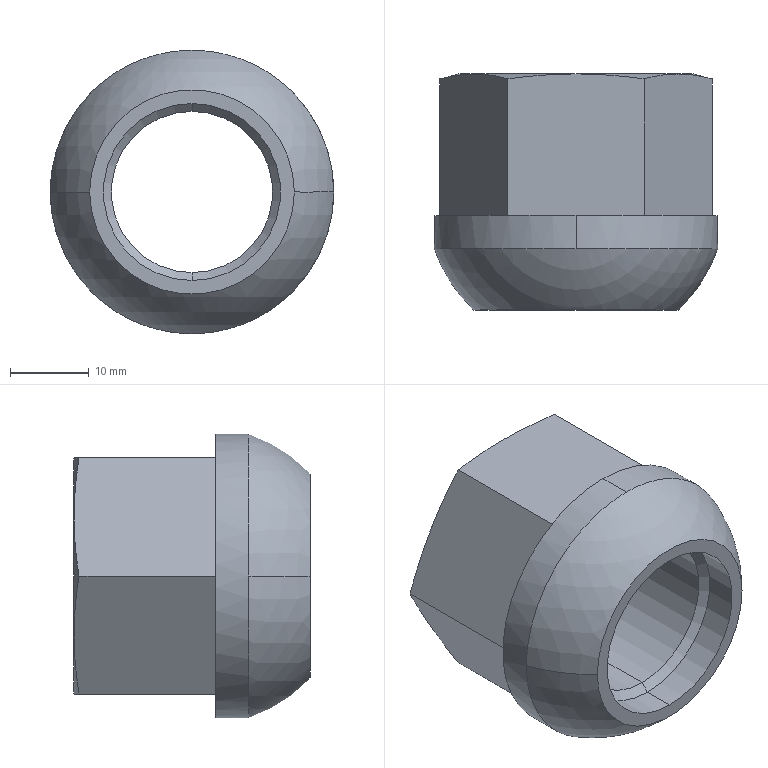Part | SolidWorks | features HoleWzd 1, ICE 1, RevCut 1, Revolution 1 | 1 solid | 21 faces | box 36 x 30 x 36 mm | volume 14362 mm3 | plane 9 | cylinder 6 | cone 4 | sphere 2 | commonest cylinder face diameters 20.5 x2 22.5 x2 36 x2
STEP:
#1=CARTESIAN_POINT('',(0.,30.,-14.928));
#2=VERTEX_POINT('',#1);
#3=CARTESIAN_POINT('',(0.,30.,14.928));
#4=VERTEX_POINT('',#3);
#5=CARTESIAN_POINT('',(0.,30.,0.));
#6=DIRECTION('',(0.,-1.,0.));
#7=DIRECTION('',(0.,0.,1.));
#8=AXIS2_PLACEMENT_3D('',#5,#6,#7);
#9=CIRCLE('',#8,14.928);
#10=EDGE_CURVE('',#2,#4,#9,.T.);
#11=ORIENTED_EDGE('',*,*,#10,.T.);
#12=CARTESIAN_POINT('',(0.,29.981,15.));
#13=VERTEX_POINT('',#12);
#14=CARTESIAN_POINT('',(0.,32.349,6.163));
#15=DIRECTION('',(0.,-0.2588,0.9659));
#16=VECTOR('',#15,1000.);
#17=LINE('',#14,#16);
#18=EDGE_CURVE('',#4,#13,#17,.T.);
#19=ORIENTED_EDGE('',*,*,#18,.T.);
#20=CARTESIAN_POINT('',(8.65,29.36,15.));
#21=VERTEX_POINT('',#20);
#22=CARTESIAN_POINT('',(0.,29.981,15.));
#23=CARTESIAN_POINT('',(1.445,29.981,15.));
#24=CARTESIAN_POINT('',(2.888,29.924,15.));
#25=CARTESIAN_POINT('',(5.771,29.71,15.));
#26=CARTESIAN_POINT('',(7.211,29.553,15.));
#27=CARTESIAN_POINT('',(8.65,29.36,15.));
#28=B_SPLINE_CURVE_WITH_KNOTS('',3,(#22,#23,#24,#25,#26,#27),.UNSPECIFIED.,.F.,.F.,(4,2,4),(0.02331,0.02767,0.03204),.UNSPECIFIED.);
#29=EDGE_CURVE('',#13,#21,#28,.T.);
#30=ORIENTED_EDGE('',*,*,#29,.T.);
#31=CARTESIAN_POINT('',(17.3,29.364,0.));
#32=VERTEX_POINT('',#31);
#33=CARTESIAN_POINT('',(8.65,29.36,15.));
#34=CARTESIAN_POINT('',(9.371,29.554,13.75));
#35=CARTESIAN_POINT('',(10.092,29.711,12.5));
#36=CARTESIAN_POINT('',(11.533,29.927,10.));
#37=CARTESIAN_POINT('',(12.254,29.984,8.75));
#38=CARTESIAN_POINT('',(13.696,29.985,6.25));
#39=CARTESIAN_POINT('',(14.417,29.928,5.));
#40=CARTESIAN_POINT('',(15.858,29.714,2.5));
#41=CARTESIAN_POINT('',(16.579,29.558,1.25));
#42=CARTESIAN_POINT('',(17.3,29.364,0.));
#43=B_SPLINE_CURVE_WITH_KNOTS('',3,(#33,#34,#35,#36,#37,#38,#39,#40,#41,#42),.UNSPECIFIED.,.F.,.F.,(4,2,2,2,4),(0.000000231,0.004329,0.008658,0.01299,0.01732),.UNSPECIFIED.);
#44=EDGE_CURVE('',#21,#32,#43,.T.);
#45=ORIENTED_EDGE('',*,*,#44,.T.);
#46=CARTESIAN_POINT('',(8.65,29.36,-15.));
#47=VERTEX_POINT('',#46);
#48=CARTESIAN_POINT('',(17.3,29.364,0.));
#49=CARTESIAN_POINT('',(16.579,29.558,-1.25));
#50=CARTESIAN_POINT('',(15.858,29.714,-2.5));
#51=CARTESIAN_POINT('',(14.417,29.928,-5.));
#52=CARTESIAN_POINT('',(13.696,29.985,-6.25));
#53=CARTESIAN_POINT('',(12.254,29.984,-8.75));
#54=CARTESIAN_POINT('',(11.533,29.927,-10.));
#55=CARTESIAN_POINT('',(10.092,29.711,-12.5));
#56=CARTESIAN_POINT('',(9.371,29.554,-13.75));
#57=CARTESIAN_POINT('',(8.65,29.36,-15.));
#58=B_SPLINE_CURVE_WITH_KNOTS('',3,(#48,#49,#50,#51,#52,#53,#54,#55,#56,#57),.UNSPECIFIED.,.F.,.F.,(4,2,2,2,4),(0.000000231,0.004329,0.008658,0.01299,0.01732),.UNSPECIFIED.);
#59=EDGE_CURVE('',#32,#47,#58,.T.);
#60=ORIENTED_EDGE('',*,*,#59,.T.);
#61=CARTESIAN_POINT('',(0.,29.981,-15.));
#62=VERTEX_POINT('',#61);
#63=CARTESIAN_POINT('',(8.65,29.36,-15.));
#64=CARTESIAN_POINT('',(7.211,29.553,-15.));
#65=CARTESIAN_POINT('',(5.771,29.71,-15.));
#66=CARTESIAN_POINT('',(2.888,29.924,-15.));
#67=CARTESIAN_POINT('',(1.445,29.981,-15.));
#68=CARTESIAN_POINT('',(0.,29.981,-15.));
#69=B_SPLINE_CURVE_WITH_KNOTS('',3,(#63,#64,#65,#66,#67,#68),.UNSPECIFIED.,.F.,.F.,(4,2,4),(0.03368,0.03804,0.04239),.UNSPECIFIED.);
#70=EDGE_CURVE('',#47,#62,#69,.T.);
#71=ORIENTED_EDGE('',*,*,#70,.T.);
#72=CARTESIAN_POINT('',(0.,32.349,-6.163));
#73=DIRECTION('',(0.,-0.2588,-0.9659));
#74=VECTOR('',#73,1000.);
#75=LINE('',#72,#74);
#76=EDGE_CURVE('',#2,#62,#75,.T.);
#77=ORIENTED_EDGE('',*,*,#76,.F.);
#78=EDGE_LOOP('',(#11,#19,#30,#45,#60,#71,#77));
#79=FACE_OUTER_BOUND('',#78,.T.);
#80=CARTESIAN_POINT('',(0.,32.349,0.));
#81=DIRECTION('',(0.,-1.,0.));
#82=DIRECTION('',(0.,0.,-1.));
#83=AXIS2_PLACEMENT_3D('',#80,#81,#82);
#84=CONICAL_SURFACE('',#83,6.163,1.309);
#85=ADVANCED_FACE('',(#79),#84,.T.);
#86=CARTESIAN_POINT('',(0.,4.96,10.25));
#87=VERTEX_POINT('',#86);
#88=CARTESIAN_POINT('',(0.,4.96,-10.25));
#89=VERTEX_POINT('',#88);
#90=CARTESIAN_POINT('',(0.,4.96,0.));
#91=DIRECTION('',(0.,-1.,0.));
#92=DIRECTION('',(0.,0.,-1.));
#93=AXIS2_PLACEMENT_3D('',#90,#91,#92);
#94=CIRCLE('',#93,10.25);
#95=EDGE_CURVE('',#87,#89,#94,.T.);
#96=ORIENTED_EDGE('',*,*,#95,.T.);
#97=CARTESIAN_POINT('',(0.,30.,-10.25));
#98=VERTEX_POINT('',#97);
#99=CARTESIAN_POINT('',(0.,30.,-10.25));
#100=DIRECTION('',(0.,1.,0.));
#101=VECTOR('',#100,1000.);
#102=LINE('',#99,#101);
#103=EDGE_CURVE('',#89,#98,#102,.T.);
#104=ORIENTED_EDGE('',*,*,#103,.T.);
#105=CARTESIAN_POINT('',(0.,30.,10.25));
#106=VERTEX_POINT('',#105);
#107=CARTESIAN_POINT('',(0.,30.,0.));
#108=DIRECTION('',(0.,1.,0.));
#109=DIRECTION('',(0.,0.,1.));
#110=AXIS2_PLACEMENT_3D('',#107,#108,#109);
#111=CIRCLE('',#110,10.25);
#112=EDGE_CURVE('',#98,#106,#111,.T.);
#113=ORIENTED_EDGE('',*,*,#112,.T.);
#114=CARTESIAN_POINT('',(0.,30.,10.25));
#115=DIRECTION('',(0.,1.,0.));
#116=VECTOR('',#115,1000.);
#117=LINE('',#114,#116);
#118=EDGE_CURVE('',#87,#106,#117,.T.);
#119=ORIENTED_EDGE('',*,*,#118,.F.);
#120=EDGE_LOOP('',(#96,#104,#113,#119));
#121=FACE_OUTER_BOUND('',#120,.T.);
#122=CARTESIAN_POINT('',(0.,30.,0.));
#123=DIRECTION('',(0.,1.,0.));
#124=DIRECTION('',(0.,0.,1.));
#125=AXIS2_PLACEMENT_3D('',#122,#123,#124);
#126=CYLINDRICAL_SURFACE('',#125,10.25);
#127=ADVANCED_FACE('',(#121),#126,.F.);
#128=ORIENTED_EDGE('',*,*,#95,.F.);
#129=CARTESIAN_POINT('',(0.,4.,11.25));
#130=VERTEX_POINT('',#129);
#131=CARTESIAN_POINT('',(0.,4.,11.25));
#132=DIRECTION('',(0.,-0.6925,0.7214));
#133=VECTOR('',#132,1000.);
#134=LINE('',#131,#133);
#135=EDGE_CURVE('',#87,#130,#134,.T.);
#136=ORIENTED_EDGE('',*,*,#135,.T.);
#137=CARTESIAN_POINT('',(0.,4.,-11.25));
#138=VERTEX_POINT('',#137);
#139=CARTESIAN_POINT('',(0.,4.,0.));
#140=DIRECTION('',(0.,1.,0.));
#141=DIRECTION('',(0.,0.,1.));
#142=AXIS2_PLACEMENT_3D('',#139,#140,#141);
#143=CIRCLE('',#142,11.25);
#144=EDGE_CURVE('',#138,#130,#143,.T.);
#145=ORIENTED_EDGE('',*,*,#144,.F.);
#146=CARTESIAN_POINT('',(0.,4.,-11.25));
#147=DIRECTION('',(0.,-0.6925,-0.7214));
#148=VECTOR('',#147,1000.);
#149=LINE('',#146,#148);
#150=EDGE_CURVE('',#89,#138,#149,.T.);
#151=ORIENTED_EDGE('',*,*,#150,.F.);
#152=EDGE_LOOP('',(#128,#136,#145,#151));
#153=FACE_OUTER_BOUND('',#152,.T.);
#154=CARTESIAN_POINT('',(0.,4.,0.));
#155=DIRECTION('',(0.,-1.,0.));
#156=DIRECTION('',(0.,0.,-1.));
#157=AXIS2_PLACEMENT_3D('',#154,#155,#156);
#158=CONICAL_SURFACE('',#157,11.25,0.8058);
#159=ADVANCED_FACE('',(#153),#158,.F.);
#160=CARTESIAN_POINT('',(0.,0.,-11.25));
#161=VERTEX_POINT('',#160);
#162=CARTESIAN_POINT('',(0.,0.,11.25));
#163=VERTEX_POINT('',#162);
#164=CARTESIAN_POINT('',(0.,0.,0.));
#165=DIRECTION('',(0.,1.,0.));
#166=DIRECTION('',(0.,0.,1.));
#167=AXIS2_PLACEMENT_3D('',#164,#165,#166);
#168=CIRCLE('',#167,11.25);
#169=EDGE_CURVE('',#161,#163,#168,.T.);
#170=ORIENTED_EDGE('',*,*,#169,.F.);
#171=CARTESIAN_POINT('',(0.,29.869,-11.25));
#172=DIRECTION('',(0.,1.,0.));
#173=VECTOR('',#172,1000.);
#174=LINE('',#171,#173);
#175=EDGE_CURVE('',#161,#138,#174,.T.);
#176=ORIENTED_EDGE('',*,*,#175,.T.);
#177=ORIENTED_EDGE('',*,*,#144,.T.);
#178=CARTESIAN_POINT('',(0.,29.869,11.25));
#179=DIRECTION('',(0.,1.,0.));
#180=VECTOR('',#179,1000.);
#181=LINE('',#178,#180);
#182=EDGE_CURVE('',#163,#130,#181,.T.);
#183=ORIENTED_EDGE('',*,*,#182,.F.);
#184=EDGE_LOOP('',(#170,#176,#177,#183));
#185=FACE_OUTER_BOUND('',#184,.T.);
#186=CARTESIAN_POINT('',(0.,29.869,0.));
#187=DIRECTION('',(0.,1.,0.));
#188=DIRECTION('',(0.,0.,1.));
#189=AXIS2_PLACEMENT_3D('',#186,#187,#188);
#190=CYLINDRICAL_SURFACE('',#189,11.25);
#191=ADVANCED_FACE('',(#185),#190,.F.);
#192=CARTESIAN_POINT('',(-13.,0.,0.));
#193=VERTEX_POINT('',#192);
#194=CARTESIAN_POINT('',(13.,0.,0.));
#195=VERTEX_POINT('',#194);
#196=CARTESIAN_POINT('',(0.,0.,0.));
#197=DIRECTION('',(0.,1.,0.));
#198=DIRECTION('',(0.,0.,1.));
#199=AXIS2_PLACEMENT_3D('',#196,#197,#198);
#200=CIRCLE('',#199,13.);
#201=EDGE_CURVE('',#193,#195,#200,.T.);
#202=ORIENTED_EDGE('',*,*,#201,.T.);
#203=CARTESIAN_POINT('',(18.,7.774,0.));
#204=VERTEX_POINT('',#203);
#205=CARTESIAN_POINT('',(0.,13.856,0.));
#206=DIRECTION('',(0.,0.,1.));
#207=DIRECTION('',(1.,0.,0.));
#208=AXIS2_PLACEMENT_3D('',#205,#206,#207);
#209=CIRCLE('',#208,19.);
#210=EDGE_CURVE('',#195,#204,#209,.T.);
#211=ORIENTED_EDGE('',*,*,#210,.T.);
#212=CARTESIAN_POINT('',(0.,7.774,18.));
#213=VERTEX_POINT('',#212);
#214=CARTESIAN_POINT('',(0.,7.774,0.));
#215=DIRECTION('',(0.,1.,0.));
#216=DIRECTION('',(0.,0.,1.));
#217=AXIS2_PLACEMENT_3D('',#214,#215,#216);
#218=CIRCLE('',#217,18.);
#219=EDGE_CURVE('',#213,#204,#218,.T.);
#220=ORIENTED_EDGE('',*,*,#219,.F.);
#221=CARTESIAN_POINT('',(-18.,7.774,0.));
#222=VERTEX_POINT('',#221);
#223=CARTESIAN_POINT('',(0.,7.774,0.));
#224=DIRECTION('',(0.,1.,0.));
#225=DIRECTION('',(0.,0.,1.));
#226=AXIS2_PLACEMENT_3D('',#223,#224,#225);
#227=CIRCLE('',#226,18.);
#228=EDGE_CURVE('',#222,#213,#227,.T.);
#229=ORIENTED_EDGE('',*,*,#228,.F.);
#230=CARTESIAN_POINT('',(0.,13.856,0.));
#231=DIRECTION('',(0.,0.,-1.));
#232=DIRECTION('',(-1.,0.,0.));
#233=AXIS2_PLACEMENT_3D('',#230,#231,#232);
#234=CIRCLE('',#233,19.);
#235=EDGE_CURVE('',#193,#222,#234,.T.);
#236=ORIENTED_EDGE('',*,*,#235,.F.);
#237=EDGE_LOOP('',(#202,#211,#220,#229,#236));
#238=FACE_OUTER_BOUND('',#237,.T.);
#239=CARTESIAN_POINT('',(0.,13.856,0.));
#240=DIRECTION('',(0.,0.,1.));
#241=DIRECTION('',(-1.,0.,0.));
#242=AXIS2_PLACEMENT_3D('',#239,#240,#241);
#243=SPHERICAL_SURFACE('',#242,19.);
#244=ADVANCED_FACE('',(#238),#243,.T.);
#245=ORIENTED_EDGE('',*,*,#219,.T.);
#246=CARTESIAN_POINT('',(0.,7.774,-18.));
#247=VERTEX_POINT('',#246);
#248=CARTESIAN_POINT('',(0.,7.774,0.));
#249=DIRECTION('',(0.,1.,0.));
#250=DIRECTION('',(0.,0.,1.));
#251=AXIS2_PLACEMENT_3D('',#248,#249,#250);
#252=CIRCLE('',#251,18.);
#253=EDGE_CURVE('',#204,#247,#252,.T.);
#254=ORIENTED_EDGE('',*,*,#253,.T.);
#255=CARTESIAN_POINT('',(0.,12.,-18.));
#256=VERTEX_POINT('',#255);
#257=CARTESIAN_POINT('',(0.,29.869,-18.));
#258=DIRECTION('',(0.,1.,0.));
#259=VECTOR('',#258,1000.);
#260=LINE('',#257,#259);
#261=EDGE_CURVE('',#247,#256,#260,.T.);
#262=ORIENTED_EDGE('',*,*,#261,.T.);
#263=CARTESIAN_POINT('',(0.,12.,18.));
#264=VERTEX_POINT('',#263);
#265=CARTESIAN_POINT('',(0.,12.,0.));
#266=DIRECTION('',(0.,-1.,0.));
#267=DIRECTION('',(0.,0.,1.));
#268=AXIS2_PLACEMENT_3D('',#265,#266,#267);
#269=CIRCLE('',#268,18.);
#270=EDGE_CURVE('',#256,#264,#269,.T.);
#271=ORIENTED_EDGE('',*,*,#270,.T.);
#272=CARTESIAN_POINT('',(0.,29.869,18.));
#273=DIRECTION('',(0.,1.,0.));
#274=VECTOR('',#273,1000.);
#275=LINE('',#272,#274);
#276=EDGE_CURVE('',#213,#264,#275,.T.);
#277=ORIENTED_EDGE('',*,*,#276,.F.);
#278=EDGE_LOOP('',(#245,#254,#262,#271,#277));
#279=FACE_OUTER_BOUND('',#278,.T.);
#280=CARTESIAN_POINT('',(0.,29.869,0.));
#281=DIRECTION('',(0.,1.,0.));
#282=DIRECTION('',(0.,0.,1.));
#283=AXIS2_PLACEMENT_3D('',#280,#281,#282);
#284=CYLINDRICAL_SURFACE('',#283,18.);
#285=ADVANCED_FACE('',(#279),#284,.T.);
#286=ORIENTED_EDGE('',*,*,#10,.F.);
#287=CARTESIAN_POINT('',(0.,30.,0.));
#288=DIRECTION('',(0.,-1.,0.));
#289=DIRECTION('',(0.,0.,1.));
#290=AXIS2_PLACEMENT_3D('',#287,#288,#289);
#291=CIRCLE('',#290,14.928);
#292=EDGE_CURVE('',#4,#2,#291,.T.);
#293=ORIENTED_EDGE('',*,*,#292,.F.);
#294=EDGE_LOOP('',(#286,#293));
#295=FACE_OUTER_BOUND('',#294,.T.);
#296=CARTESIAN_POINT('',(0.,30.,0.));
#297=DIRECTION('',(0.,1.,0.));
#298=DIRECTION('',(0.,0.,1.));
#299=AXIS2_PLACEMENT_3D('',#296,#297,#298);
#300=CIRCLE('',#299,10.25);
#301=EDGE_CURVE('',#106,#98,#300,.T.);
#302=ORIENTED_EDGE('',*,*,#301,.F.);
#303=ORIENTED_EDGE('',*,*,#112,.F.);
#304=EDGE_LOOP('',(#302,#303));
#305=FACE_BOUND('',#304,.T.);
#306=CARTESIAN_POINT('',(-18.,30.,0.));
#307=DIRECTION('',(0.,1.,0.));
#308=DIRECTION('',(0.,0.,1.));
#309=AXIS2_PLACEMENT_3D('',#306,#307,#308);
#310=PLANE('',#309);
#311=ADVANCED_FACE('',(#295,#305),#310,.T.);
#312=ORIENTED_EDGE('',*,*,#261,.F.);
#313=CARTESIAN_POINT('',(0.,7.774,0.));
#314=DIRECTION('',(0.,1.,0.));
#315=DIRECTION('',(0.,0.,1.));
#316=AXIS2_PLACEMENT_3D('',#313,#314,#315);
#317=CIRCLE('',#316,18.);
#318=EDGE_CURVE('',#247,#222,#317,.T.);
#319=ORIENTED_EDGE('',*,*,#318,.T.);
#320=ORIENTED_EDGE('',*,*,#228,.T.);
#321=ORIENTED_EDGE('',*,*,#276,.T.);
#322=CARTESIAN_POINT('',(0.,12.,0.));
#323=DIRECTION('',(0.,-1.,0.));
#324=DIRECTION('',(0.,0.,1.));
#325=AXIS2_PLACEMENT_3D('',#322,#323,#324);
#326=CIRCLE('',#325,18.);
#327=EDGE_CURVE('',#264,#256,#326,.T.);
#328=ORIENTED_EDGE('',*,*,#327,.T.);
#329=EDGE_LOOP('',(#312,#319,#320,#321,#328));
#330=FACE_OUTER_BOUND('',#329,.T.);
#331=CARTESIAN_POINT('',(0.,29.869,0.));
#332=DIRECTION('',(0.,1.,0.));
#333=DIRECTION('',(0.,0.,1.));
#334=AXIS2_PLACEMENT_3D('',#331,#332,#333);
#335=CYLINDRICAL_SURFACE('',#334,18.);
#336=ADVANCED_FACE('',(#330),#335,.T.);
#337=ORIENTED_EDGE('',*,*,#210,.F.);
#338=CARTESIAN_POINT('',(0.,0.,0.));
#339=DIRECTION('',(0.,1.,0.));
#340=DIRECTION('',(0.,0.,1.));
#341=AXIS2_PLACEMENT_3D('',#338,#339,#340);
#342=CIRCLE('',#341,13.);
#343=EDGE_CURVE('',#195,#193,#342,.T.);
#344=ORIENTED_EDGE('',*,*,#343,.T.);
#345=ORIENTED_EDGE('',*,*,#235,.T.);
#346=ORIENTED_EDGE('',*,*,#318,.F.);
#347=ORIENTED_EDGE('',*,*,#253,.F.);
#348=EDGE_LOOP('',(#337,#344,#345,#346,#347));
#349=FACE_OUTER_BOUND('',#348,.T.);
#350=CARTESIAN_POINT('',(0.,13.856,0.));
#351=DIRECTION('',(0.,0.,1.));
#352=DIRECTION('',(-1.,0.,0.));
#353=AXIS2_PLACEMENT_3D('',#350,#351,#352);
#354=SPHERICAL_SURFACE('',#353,19.);
#355=ADVANCED_FACE('',(#349),#354,.T.);
#356=CARTESIAN_POINT('',(0.,0.,0.));
#357=DIRECTION('',(0.,1.,0.));
#358=DIRECTION('',(0.,0.,1.));
#359=AXIS2_PLACEMENT_3D('',#356,#357,#358);
#360=CIRCLE('',#359,11.25);
#361=EDGE_CURVE('',#163,#161,#360,.T.);
#362=ORIENTED_EDGE('',*,*,#361,.T.);
#363=ORIENTED_EDGE('',*,*,#169,.T.);
#364=EDGE_LOOP('',(#362,#363));
#365=FACE_BOUND('',#364,.T.);
#366=ORIENTED_EDGE('',*,*,#201,.F.);
#367=ORIENTED_EDGE('',*,*,#343,.F.);
#368=EDGE_LOOP('',(#366,#367));
#369=FACE_OUTER_BOUND('',#368,.T.);
#370=CARTESIAN_POINT('',(-13.,0.,0.));
#371=DIRECTION('',(0.,-1.,0.));
#372=DIRECTION('',(0.,0.,-1.));
#373=AXIS2_PLACEMENT_3D('',#370,#371,#372);
#374=PLANE('',#373);
#375=ADVANCED_FACE('',(#365,#369),#374,.T.);
#376=ORIENTED_EDGE('',*,*,#175,.F.);
#377=ORIENTED_EDGE('',*,*,#361,.F.);
#378=ORIENTED_EDGE('',*,*,#182,.T.);
#379=CARTESIAN_POINT('',(0.,4.,0.));
#380=DIRECTION('',(0.,1.,0.));
#381=DIRECTION('',(0.,0.,1.));
#382=AXIS2_PLACEMENT_3D('',#379,#380,#381);
#383=CIRCLE('',#382,11.25);
#384=EDGE_CURVE('',#130,#138,#383,.T.);
#385=ORIENTED_EDGE('',*,*,#384,.T.);
#386=EDGE_LOOP('',(#376,#377,#378,#385));
#387=FACE_OUTER_BOUND('',#386,.T.);
#388=CARTESIAN_POINT('',(0.,29.869,0.));
#389=DIRECTION('',(0.,1.,0.));
#390=DIRECTION('',(0.,0.,1.));
#391=AXIS2_PLACEMENT_3D('',#388,#389,#390);
#392=CYLINDRICAL_SURFACE('',#391,11.25);
#393=ADVANCED_FACE('',(#387),#392,.F.);
#394=ORIENTED_EDGE('',*,*,#135,.F.);
#395=CARTESIAN_POINT('',(0.,4.96,0.));
#396=DIRECTION('',(0.,-1.,0.));
#397=DIRECTION('',(0.,0.,-1.));
#398=AXIS2_PLACEMENT_3D('',#395,#396,#397);
#399=CIRCLE('',#398,10.25);
#400=EDGE_CURVE('',#89,#87,#399,.T.);
#401=ORIENTED_EDGE('',*,*,#400,.F.);
#402=ORIENTED_EDGE('',*,*,#150,.T.);
#403=ORIENTED_EDGE('',*,*,#384,.F.);
#404=EDGE_LOOP('',(#394,#401,#402,#403));
#405=FACE_OUTER_BOUND('',#404,.T.);
#406=CARTESIAN_POINT('',(0.,4.,0.));
#407=DIRECTION('',(0.,-1.,0.));
#408=DIRECTION('',(0.,0.,-1.));
#409=AXIS2_PLACEMENT_3D('',#406,#407,#408);
#410=CONICAL_SURFACE('',#409,11.25,0.8058);
#411=ADVANCED_FACE('',(#405),#410,.F.);
#412=ORIENTED_EDGE('',*,*,#103,.F.);
#413=ORIENTED_EDGE('',*,*,#400,.T.);
#414=ORIENTED_EDGE('',*,*,#118,.T.);
#415=ORIENTED_EDGE('',*,*,#301,.T.);
#416=EDGE_LOOP('',(#412,#413,#414,#415));
#417=FACE_OUTER_BOUND('',#416,.T.);
#418=CARTESIAN_POINT('',(0.,30.,0.));
#419=DIRECTION('',(0.,1.,0.));
#420=DIRECTION('',(0.,0.,1.));
#421=AXIS2_PLACEMENT_3D('',#418,#419,#420);
#422=CYLINDRICAL_SURFACE('',#421,10.25);
#423=ADVANCED_FACE('',(#417),#422,.F.);
#424=ORIENTED_EDGE('',*,*,#327,.F.);
#425=ORIENTED_EDGE('',*,*,#270,.F.);
#426=EDGE_LOOP('',(#424,#425));
#427=FACE_OUTER_BOUND('',#426,.T.);
#428=CARTESIAN_POINT('',(8.65,12.,-15.));
#429=VERTEX_POINT('',#428);
#430=CARTESIAN_POINT('',(-8.65,12.,-15.));
#431=VERTEX_POINT('',#430);
#432=CARTESIAN_POINT('',(-8.65,12.,-15.));
#433=DIRECTION('',(-1.,0.,0.));
#434=VECTOR('',#433,1000.);
#435=LINE('',#432,#434);
#436=EDGE_CURVE('',#429,#431,#435,.T.);
#437=ORIENTED_EDGE('',*,*,#436,.F.);
#438=CARTESIAN_POINT('',(17.3,12.,0.));
#439=VERTEX_POINT('',#438);
#440=CARTESIAN_POINT('',(8.65,12.,-15.));
#441=DIRECTION('',(-0.4996,0.,-0.8663));
#442=VECTOR('',#441,1000.);
#443=LINE('',#440,#442);
#444=EDGE_CURVE('',#439,#429,#443,.T.);
#445=ORIENTED_EDGE('',*,*,#444,.F.);
#446=CARTESIAN_POINT('',(8.65,12.,15.));
#447=VERTEX_POINT('',#446);
#448=CARTESIAN_POINT('',(8.65,12.,15.));
#449=DIRECTION('',(0.4996,0.,-0.8663));
#450=VECTOR('',#449,1000.);
#451=LINE('',#448,#450);
#452=EDGE_CURVE('',#447,#439,#451,.T.);
#453=ORIENTED_EDGE('',*,*,#452,.F.);
#454=CARTESIAN_POINT('',(-8.65,12.,15.));
#455=VERTEX_POINT('',#454);
#456=CARTESIAN_POINT('',(-8.65,12.,15.));
#457=DIRECTION('',(1.,0.,0.));
#458=VECTOR('',#457,1000.);
#459=LINE('',#456,#458);
#460=EDGE_CURVE('',#455,#447,#459,.T.);
#461=ORIENTED_EDGE('',*,*,#460,.F.);
#462=CARTESIAN_POINT('',(-17.3,12.,0.));
#463=VERTEX_POINT('',#462);
#464=CARTESIAN_POINT('',(-8.65,12.,15.));
#465=DIRECTION('',(0.4996,0.,0.8663));
#466=VECTOR('',#465,1000.);
#467=LINE('',#464,#466);
#468=EDGE_CURVE('',#463,#455,#467,.T.);
#469=ORIENTED_EDGE('',*,*,#468,.F.);
#470=CARTESIAN_POINT('',(-8.65,12.,-15.));
#471=DIRECTION('',(-0.4996,0.,0.8663));
#472=VECTOR('',#471,1000.);
#473=LINE('',#470,#472);
#474=EDGE_CURVE('',#431,#463,#473,.T.);
#475=ORIENTED_EDGE('',*,*,#474,.F.);
#476=EDGE_LOOP('',(#437,#445,#453,#461,#469,#475));
#477=FACE_BOUND('',#476,.T.);
#478=CARTESIAN_POINT('',(0.,12.,0.));
#479=DIRECTION('',(0.,1.,0.));
#480=DIRECTION('',(0.,0.,1.));
#481=AXIS2_PLACEMENT_3D('',#478,#479,#480);
#482=PLANE('',#481);
#483=ADVANCED_FACE('',(#427,#477),#482,.T.);
#484=CARTESIAN_POINT('',(-8.65,29.36,-15.));
#485=VERTEX_POINT('',#484);
#486=CARTESIAN_POINT('',(-17.3,29.364,0.));
#487=VERTEX_POINT('',#486);
#488=CARTESIAN_POINT('',(-8.65,29.36,-15.));
#489=CARTESIAN_POINT('',(-9.371,29.554,-13.75));
#490=CARTESIAN_POINT('',(-10.092,29.711,-12.5));
#491=CARTESIAN_POINT('',(-11.533,29.927,-10.));
#492=CARTESIAN_POINT('',(-12.254,29.984,-8.75));
#493=CARTESIAN_POINT('',(-13.696,29.985,-6.25));
#494=CARTESIAN_POINT('',(-14.417,29.928,-5.));
#495=CARTESIAN_POINT('',(-15.858,29.714,-2.5));
#496=CARTESIAN_POINT('',(-16.579,29.558,-1.25));
#497=CARTESIAN_POINT('',(-17.3,29.364,0.));
#498=B_SPLINE_CURVE_WITH_KNOTS('',3,(#488,#489,#490,#491,#492,#493,#494,#495,#496,#497),.UNSPECIFIED.,.F.,.F.,(4,2,2,2,4),(0.000000231,0.004329,0.008658,0.01299,0.01732),.UNSPECIFIED.);
#499=EDGE_CURVE('',#485,#487,#498,.T.);
#500=ORIENTED_EDGE('',*,*,#499,.F.);
#501=CARTESIAN_POINT('',(-8.65,12.,-15.));
#502=DIRECTION('',(0.,1.,0.));
#503=VECTOR('',#502,1000.);
#504=LINE('',#501,#503);
#505=EDGE_CURVE('',#431,#485,#504,.T.);
#506=ORIENTED_EDGE('',*,*,#505,.F.);
#507=ORIENTED_EDGE('',*,*,#474,.T.);
#508=CARTESIAN_POINT('',(-17.3,12.,0.));
#509=DIRECTION('',(0.,1.,0.));
#510=VECTOR('',#509,1000.);
#511=LINE('',#508,#510);
#512=EDGE_CURVE('',#463,#487,#511,.T.);
#513=ORIENTED_EDGE('',*,*,#512,.T.);
#514=EDGE_LOOP('',(#500,#506,#507,#513));
#515=FACE_OUTER_BOUND('',#514,.T.);
#516=CARTESIAN_POINT('',(-8.65,12.,-15.));
#517=DIRECTION('',(-0.8663,0.,-0.4996));
#518=DIRECTION('',(-0.4996,0.,0.8663));
#519=AXIS2_PLACEMENT_3D('',#516,#517,#518);
#520=PLANE('',#519);
#521=ADVANCED_FACE('',(#515),#520,.T.);
#522=ORIENTED_EDGE('',*,*,#70,.F.);
#523=CARTESIAN_POINT('',(8.65,12.,-15.));
#524=DIRECTION('',(0.,1.,0.));
#525=VECTOR('',#524,1000.);
#526=LINE('',#523,#525);
#527=EDGE_CURVE('',#429,#47,#526,.T.);
#528=ORIENTED_EDGE('',*,*,#527,.F.);
#529=ORIENTED_EDGE('',*,*,#436,.T.);
#530=ORIENTED_EDGE('',*,*,#505,.T.);
#531=CARTESIAN_POINT('',(0.,29.981,-15.));
#532=CARTESIAN_POINT('',(-1.44,29.981,-15.));
#533=CARTESIAN_POINT('',(-2.881,29.924,-15.));
#534=CARTESIAN_POINT('',(-5.766,29.71,-15.));
#535=CARTESIAN_POINT('',(-7.213,29.553,-15.));
#536=CARTESIAN_POINT('',(-8.65,29.36,-15.));
#537=B_SPLINE_CURVE_WITH_KNOTS('',3,(#531,#532,#533,#534,#535,#536),.UNSPECIFIED.,.F.,.F.,(4,2,4),(0.04239,0.04673,0.05107),.UNSPECIFIED.);
#538=EDGE_CURVE('',#62,#485,#537,.T.);
#539=ORIENTED_EDGE('',*,*,#538,.F.);
#540=EDGE_LOOP('',(#522,#528,#529,#530,#539));
#541=FACE_OUTER_BOUND('',#540,.T.);
#542=CARTESIAN_POINT('',(-8.65,12.,-15.));
#543=DIRECTION('',(0.,0.,-1.));
#544=DIRECTION('',(-1.,0.,0.));
#545=AXIS2_PLACEMENT_3D('',#542,#543,#544);
#546=PLANE('',#545);
#547=ADVANCED_FACE('',(#541),#546,.T.);
#548=ORIENTED_EDGE('',*,*,#59,.F.);
#549=CARTESIAN_POINT('',(17.3,12.,0.));
#550=DIRECTION('',(0.,1.,0.));
#551=VECTOR('',#550,1000.);
#552=LINE('',#549,#551);
#553=EDGE_CURVE('',#439,#32,#552,.T.);
#554=ORIENTED_EDGE('',*,*,#553,.F.);
#555=ORIENTED_EDGE('',*,*,#444,.T.);
#556=ORIENTED_EDGE('',*,*,#527,.T.);
#557=EDGE_LOOP('',(#548,#554,#555,#556));
#558=FACE_OUTER_BOUND('',#557,.T.);
#559=CARTESIAN_POINT('',(8.65,12.,-15.));
#560=DIRECTION('',(0.8663,0.,-0.4996));
#561=DIRECTION('',(-0.4996,0.,-0.8663));
#562=AXIS2_PLACEMENT_3D('',#559,#560,#561);
#563=PLANE('',#562);
#564=ADVANCED_FACE('',(#558),#563,.T.);
#565=ORIENTED_EDGE('',*,*,#44,.F.);
#566=CARTESIAN_POINT('',(8.65,12.,15.));
#567=DIRECTION('',(0.,1.,0.));
#568=VECTOR('',#567,1000.);
#569=LINE('',#566,#568);
#570=EDGE_CURVE('',#447,#21,#569,.T.);
#571=ORIENTED_EDGE('',*,*,#570,.F.);
#572=ORIENTED_EDGE('',*,*,#452,.T.);
#573=ORIENTED_EDGE('',*,*,#553,.T.);
#574=EDGE_LOOP('',(#565,#571,#572,#573));
#575=FACE_OUTER_BOUND('',#574,.T.);
#576=CARTESIAN_POINT('',(8.65,12.,15.));
#577=DIRECTION('',(0.8663,0.,0.4996));
#578=DIRECTION('',(0.4996,0.,-0.8663));
#579=AXIS2_PLACEMENT_3D('',#576,#577,#578);
#580=PLANE('',#579);
#581=ADVANCED_FACE('',(#575),#580,.T.);
#582=CARTESIAN_POINT('',(-8.65,29.36,15.));
#583=VERTEX_POINT('',#582);
#584=CARTESIAN_POINT('',(-8.65,29.36,15.));
#585=CARTESIAN_POINT('',(-7.213,29.553,15.));
#586=CARTESIAN_POINT('',(-5.766,29.71,15.));
#587=CARTESIAN_POINT('',(-2.881,29.924,15.));
#588=CARTESIAN_POINT('',(-1.44,29.981,15.));
#589=CARTESIAN_POINT('',(0.,29.981,15.));
#590=B_SPLINE_CURVE_WITH_KNOTS('',3,(#584,#585,#586,#587,#588,#589),.UNSPECIFIED.,.F.,.F.,(4,2,4),(0.01462,0.01897,0.02331),.UNSPECIFIED.);
#591=EDGE_CURVE('',#583,#13,#590,.T.);
#592=ORIENTED_EDGE('',*,*,#591,.F.);
#593=CARTESIAN_POINT('',(-8.65,12.,15.));
#594=DIRECTION('',(0.,1.,0.));
#595=VECTOR('',#594,1000.);
#596=LINE('',#593,#595);
#597=EDGE_CURVE('',#455,#583,#596,.T.);
#598=ORIENTED_EDGE('',*,*,#597,.F.);
#599=ORIENTED_EDGE('',*,*,#460,.T.);
#600=ORIENTED_EDGE('',*,*,#570,.T.);
#601=ORIENTED_EDGE('',*,*,#29,.F.);
#602=EDGE_LOOP('',(#592,#598,#599,#600,#601));
#603=FACE_OUTER_BOUND('',#602,.T.);
#604=CARTESIAN_POINT('',(-8.65,12.,15.));
#605=DIRECTION('',(0.,0.,1.));
#606=DIRECTION('',(1.,0.,0.));
#607=AXIS2_PLACEMENT_3D('',#604,#605,#606);
#608=PLANE('',#607);
#609=ADVANCED_FACE('',(#603),#608,.T.);
#610=CARTESIAN_POINT('',(-17.3,29.364,0.));
#611=CARTESIAN_POINT('',(-16.579,29.558,1.25));
#612=CARTESIAN_POINT('',(-15.858,29.714,2.5));
#613=CARTESIAN_POINT('',(-14.417,29.928,5.));
#614=CARTESIAN_POINT('',(-13.696,29.985,6.25));
#615=CARTESIAN_POINT('',(-12.254,29.984,8.75));
#616=CARTESIAN_POINT('',(-11.533,29.927,10.));
#617=CARTESIAN_POINT('',(-10.092,29.711,12.5));
#618=CARTESIAN_POINT('',(-9.371,29.554,13.75));
#619=CARTESIAN_POINT('',(-8.65,29.36,15.));
#620=B_SPLINE_CURVE_WITH_KNOTS('',3,(#610,#611,#612,#613,#614,#615,#616,#617,#618,#619),.UNSPECIFIED.,.F.,.F.,(4,2,2,2,4),(0.000000231,0.004329,0.008658,0.01299,0.01732),.UNSPECIFIED.);
#621=EDGE_CURVE('',#487,#583,#620,.T.);
#622=ORIENTED_EDGE('',*,*,#621,.F.);
#623=ORIENTED_EDGE('',*,*,#512,.F.);
#624=ORIENTED_EDGE('',*,*,#468,.T.);
#625=ORIENTED_EDGE('',*,*,#597,.T.);
#626=EDGE_LOOP('',(#622,#623,#624,#625));
#627=FACE_OUTER_BOUND('',#626,.T.);
#628=CARTESIAN_POINT('',(-8.65,12.,15.));
#629=DIRECTION('',(-0.8663,0.,0.4996));
#630=DIRECTION('',(0.4996,0.,0.8663));
#631=AXIS2_PLACEMENT_3D('',#628,#629,#630);
#632=PLANE('',#631);
#633=ADVANCED_FACE('',(#627),#632,.T.);
#634=ORIENTED_EDGE('',*,*,#18,.F.);
#635=ORIENTED_EDGE('',*,*,#292,.T.);
#636=ORIENTED_EDGE('',*,*,#76,.T.);
#637=ORIENTED_EDGE('',*,*,#538,.T.);
#638=ORIENTED_EDGE('',*,*,#499,.T.);
#639=ORIENTED_EDGE('',*,*,#621,.T.);
#640=ORIENTED_EDGE('',*,*,#591,.T.);
#641=EDGE_LOOP('',(#634,#635,#636,#637,#638,#639,#640));
#642=FACE_OUTER_BOUND('',#641,.T.);
#643=CARTESIAN_POINT('',(0.,32.349,0.));
#644=DIRECTION('',(0.,-1.,0.));
#645=DIRECTION('',(0.,0.,-1.));
#646=AXIS2_PLACEMENT_3D('',#643,#644,#645);
#647=CONICAL_SURFACE('',#646,6.163,1.309);
#648=ADVANCED_FACE('',(#642),#647,.T.);
#649=CLOSED_SHELL('',(#85,#127,#159,#191,#244,#285,#311,#336,#355,#375,#393,#411,#423,#483,#521,#547,#564,#581,#609,#633,#648));
#650=MANIFOLD_SOLID_BREP('',#649);
#651=CARTESIAN_POINT('',(0.,0.,0.));
#652=DIRECTION('',(0.,0.,1.));
#653=DIRECTION('',(1.,0.,0.));
#654=AXIS2_PLACEMENT_3D('',#651,#652,#653);
#655=(LENGTH_UNIT()NAMED_UNIT(*)SI_UNIT(.MILLI.,.METRE.));
#656=UNCERTAINTY_MEASURE_WITH_UNIT(LENGTH_MEASURE(0.00001),#655,'','');
#657=(NAMED_UNIT(*)PLANE_ANGLE_UNIT()SI_UNIT($,.RADIAN.));
#658=(NAMED_UNIT(*)SI_UNIT($,.STERADIAN.)SOLID_ANGLE_UNIT());
#659=(GEOMETRIC_REPRESENTATION_CONTEXT(3)GLOBAL_UNCERTAINTY_ASSIGNED_CONTEXT((#656))GLOBAL_UNIT_ASSIGNED_CONTEXT((#655,#657,#658))REPRESENTATION_CONTEXT('',''));
#660=ADVANCED_BREP_SHAPE_REPRESENTATION('',(#650,#654),#659);